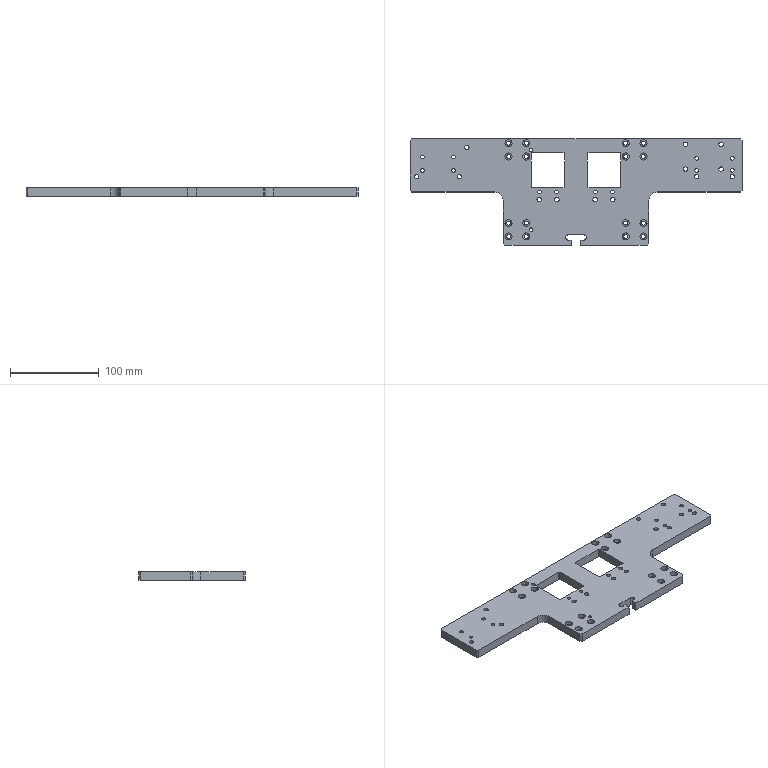Part | 1 solid | 117 faces | box 374 x 120 x 10 mm | volume 282006 mm3 | cylinder 71 | plane 46 | commonest cylinder face diameters 4.5 x16 8 x16 5 x13 4.2 x12 2 x8 4 x2